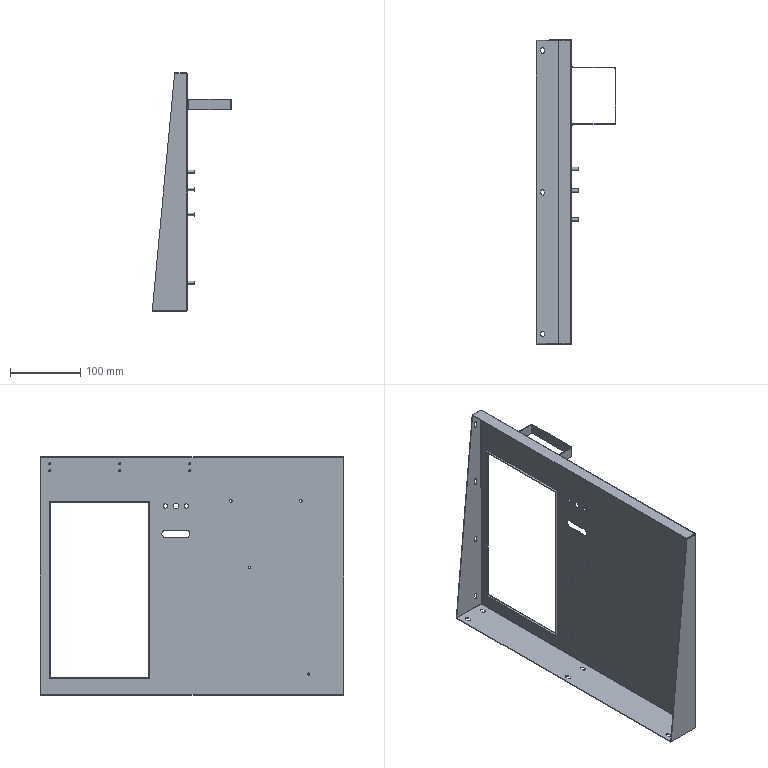Part | STEP file | RJWD-DY-0114_X2_75356C145B89_10 | 10 solids | 226 faces | box 113.5 x 434 x 340 mm | volume 170020 mm3 | plane 117 | cylinder 100 | spline 9 | commonest cylinder face diameters 2.5 x16 3 x16 5.4 x16 4.5 x12 4 x8 5 x8